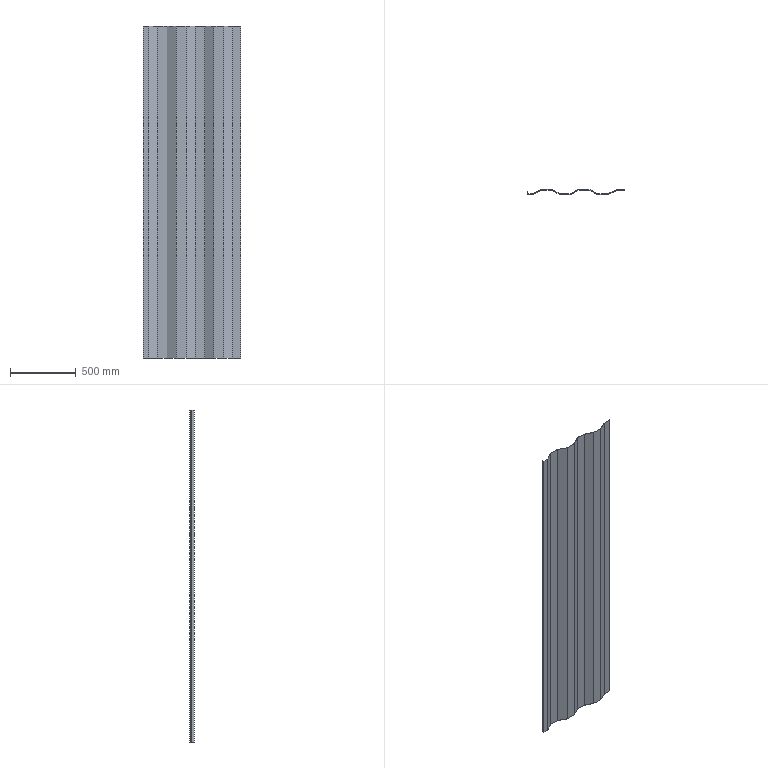Part | SolidWorks | features ExtruThin 1 | 1 solid | 28 faces | box 742 x 37.696 x 2530 mm | volume 4059329 mm3 | plane 28
STEP:
#1=CARTESIAN_POINT('',(679.865,31.696,0.));
#2=VERTEX_POINT('',#1);
#3=CARTESIAN_POINT('',(742.,31.696,0.));
#4=VERTEX_POINT('',#3);
#5=CARTESIAN_POINT('',(679.865,31.696,0.));
#6=DIRECTION('',(1.,0.,0.));
#7=VECTOR('',#6,1000.);
#8=LINE('',#5,#7);
#9=EDGE_CURVE('',#2,#4,#8,.T.);
#10=ORIENTED_EDGE('',*,*,#9,.T.);
#11=CARTESIAN_POINT('',(742.,31.696,2530.));
#12=VERTEX_POINT('',#11);
#13=CARTESIAN_POINT('',(742.,31.696,2530.));
#14=DIRECTION('',(0.,0.,-1.));
#15=VECTOR('',#14,1000.);
#16=LINE('',#13,#15);
#17=EDGE_CURVE('',#12,#4,#16,.T.);
#18=ORIENTED_EDGE('',*,*,#17,.F.);
#19=CARTESIAN_POINT('',(679.865,31.696,2530.));
#20=VERTEX_POINT('',#19);
#21=CARTESIAN_POINT('',(679.865,31.696,2530.));
#22=DIRECTION('',(1.,0.,0.));
#23=VECTOR('',#22,1000.);
#24=LINE('',#21,#23);
#25=EDGE_CURVE('',#20,#12,#24,.T.);
#26=ORIENTED_EDGE('',*,*,#25,.F.);
#27=CARTESIAN_POINT('',(679.865,31.696,2530.));
#28=DIRECTION('',(0.,0.,-1.));
#29=VECTOR('',#28,1000.);
#30=LINE('',#27,#29);
#31=EDGE_CURVE('',#20,#2,#30,.T.);
#32=ORIENTED_EDGE('',*,*,#31,.T.);
#33=EDGE_LOOP('',(#10,#18,#26,#32));
#34=FACE_OUTER_BOUND('',#33,.T.);
#35=CARTESIAN_POINT('',(679.865,31.696,2530.));
#36=DIRECTION('',(0.,1.,0.));
#37=DIRECTION('',(0.,0.,1.));
#38=AXIS2_PLACEMENT_3D('',#35,#36,#37);
#39=PLANE('',#38);
#40=ADVANCED_FACE('',(#34),#39,.F.);
#41=CARTESIAN_POINT('',(742.,33.696,0.));
#42=VERTEX_POINT('',#41);
#43=CARTESIAN_POINT('',(742.,33.696,0.));
#44=DIRECTION('',(0.,-1.,0.));
#45=VECTOR('',#44,1000.);
#46=LINE('',#43,#45);
#47=EDGE_CURVE('',#42,#4,#46,.T.);
#48=ORIENTED_EDGE('',*,*,#47,.F.);
#49=CARTESIAN_POINT('',(742.,33.696,2530.));
#50=VERTEX_POINT('',#49);
#51=CARTESIAN_POINT('',(742.,33.696,2530.));
#52=DIRECTION('',(0.,0.,-1.));
#53=VECTOR('',#52,1000.);
#54=LINE('',#51,#53);
#55=EDGE_CURVE('',#50,#42,#54,.T.);
#56=ORIENTED_EDGE('',*,*,#55,.F.);
#57=CARTESIAN_POINT('',(742.,33.696,2530.));
#58=DIRECTION('',(0.,-1.,0.));
#59=VECTOR('',#58,1000.);
#60=LINE('',#57,#59);
#61=EDGE_CURVE('',#50,#12,#60,.T.);
#62=ORIENTED_EDGE('',*,*,#61,.T.);
#63=ORIENTED_EDGE('',*,*,#17,.T.);
#64=EDGE_LOOP('',(#48,#56,#62,#63));
#65=FACE_OUTER_BOUND('',#64,.T.);
#66=CARTESIAN_POINT('',(742.,33.696,2530.));
#67=DIRECTION('',(1.,0.,0.));
#68=DIRECTION('',(0.,0.,-1.));
#69=AXIS2_PLACEMENT_3D('',#66,#67,#68);
#70=PLANE('',#69);
#71=ADVANCED_FACE('',(#65),#70,.T.);
#72=CARTESIAN_POINT('',(679.422,33.696,0.));
#73=VERTEX_POINT('',#72);
#74=CARTESIAN_POINT('',(679.865,33.696,0.));
#75=DIRECTION('',(1.,0.,0.));
#76=VECTOR('',#75,1000.);
#77=LINE('',#74,#76);
#78=EDGE_CURVE('',#73,#42,#77,.T.);
#79=ORIENTED_EDGE('',*,*,#78,.F.);
#80=CARTESIAN_POINT('',(679.422,33.696,2530.));
#81=VERTEX_POINT('',#80);
#82=CARTESIAN_POINT('',(679.422,33.696,2530.));
#83=DIRECTION('',(0.,0.,-1.));
#84=VECTOR('',#83,1000.);
#85=LINE('',#82,#84);
#86=EDGE_CURVE('',#81,#73,#85,.T.);
#87=ORIENTED_EDGE('',*,*,#86,.F.);
#88=CARTESIAN_POINT('',(679.865,33.696,2530.));
#89=DIRECTION('',(1.,0.,0.));
#90=VECTOR('',#89,1000.);
#91=LINE('',#88,#90);
#92=EDGE_CURVE('',#81,#50,#91,.T.);
#93=ORIENTED_EDGE('',*,*,#92,.T.);
#94=ORIENTED_EDGE('',*,*,#55,.T.);
#95=EDGE_LOOP('',(#79,#87,#93,#94));
#96=FACE_OUTER_BOUND('',#95,.T.);
#97=CARTESIAN_POINT('',(679.865,33.696,2530.));
#98=DIRECTION('',(0.,1.,0.));
#99=DIRECTION('',(0.,0.,1.));
#100=AXIS2_PLACEMENT_3D('',#97,#98,#99);
#101=PLANE('',#100);
#102=ADVANCED_FACE('',(#96),#101,.T.);
#103=CARTESIAN_POINT('',(611.449,2.,0.));
#104=VERTEX_POINT('',#103);
#105=CARTESIAN_POINT('',(611.047,1.813,0.));
#106=DIRECTION('',(0.9063,0.4226,0.));
#107=VECTOR('',#106,1000.);
#108=LINE('',#105,#107);
#109=EDGE_CURVE('',#104,#73,#108,.T.);
#110=ORIENTED_EDGE('',*,*,#109,.F.);
#111=CARTESIAN_POINT('',(611.449,2.,2530.));
#112=VERTEX_POINT('',#111);
#113=CARTESIAN_POINT('',(611.449,2.,2530.));
#114=DIRECTION('',(0.,0.,-1.));
#115=VECTOR('',#114,1000.);
#116=LINE('',#113,#115);
#117=EDGE_CURVE('',#112,#104,#116,.T.);
#118=ORIENTED_EDGE('',*,*,#117,.F.);
#119=CARTESIAN_POINT('',(611.047,1.813,2530.));
#120=DIRECTION('',(0.9063,0.4226,0.));
#121=VECTOR('',#120,1000.);
#122=LINE('',#119,#121);
#123=EDGE_CURVE('',#112,#81,#122,.T.);
#124=ORIENTED_EDGE('',*,*,#123,.T.);
#125=ORIENTED_EDGE('',*,*,#86,.T.);
#126=EDGE_LOOP('',(#110,#118,#124,#125));
#127=FACE_OUTER_BOUND('',#126,.T.);
#128=CARTESIAN_POINT('',(611.047,1.813,2530.));
#129=DIRECTION('',(-0.4226,0.9063,0.));
#130=DIRECTION('',(-0.9063,-0.4226,0.));
#131=AXIS2_PLACEMENT_3D('',#128,#129,#130);
#132=PLANE('',#131);
#133=ADVANCED_FACE('',(#127),#132,.T.);
#134=CARTESIAN_POINT('',(537.386,2.,0.));
#135=VERTEX_POINT('',#134);
#136=CARTESIAN_POINT('',(536.892,2.,0.));
#137=DIRECTION('',(1.,0.,0.));
#138=VECTOR('',#137,1000.);
#139=LINE('',#136,#138);
#140=EDGE_CURVE('',#135,#104,#139,.T.);
#141=ORIENTED_EDGE('',*,*,#140,.F.);
#142=CARTESIAN_POINT('',(537.386,2.,2530.));
#143=VERTEX_POINT('',#142);
#144=CARTESIAN_POINT('',(537.386,2.,2530.));
#145=DIRECTION('',(0.,0.,-1.));
#146=VECTOR('',#145,1000.);
#147=LINE('',#144,#146);
#148=EDGE_CURVE('',#143,#135,#147,.T.);
#149=ORIENTED_EDGE('',*,*,#148,.F.);
#150=CARTESIAN_POINT('',(536.892,2.,2530.));
#151=DIRECTION('',(1.,0.,0.));
#152=VECTOR('',#151,1000.);
#153=LINE('',#150,#152);
#154=EDGE_CURVE('',#143,#112,#153,.T.);
#155=ORIENTED_EDGE('',*,*,#154,.T.);
#156=ORIENTED_EDGE('',*,*,#117,.T.);
#157=EDGE_LOOP('',(#141,#149,#155,#156));
#158=FACE_OUTER_BOUND('',#157,.T.);
#159=CARTESIAN_POINT('',(536.892,2.,2530.));
#160=DIRECTION('',(0.,1.,0.));
#161=DIRECTION('',(0.,0.,1.));
#162=AXIS2_PLACEMENT_3D('',#159,#160,#161);
#163=PLANE('',#162);
#164=ADVANCED_FACE('',(#158),#163,.T.);
#165=CARTESIAN_POINT('',(469.412,37.696,0.));
#166=VERTEX_POINT('',#165);
#167=CARTESIAN_POINT('',(469.849,37.467,0.));
#168=DIRECTION('',(0.8853,-0.4649,0.));
#169=VECTOR('',#168,1000.);
#170=LINE('',#167,#169);
#171=EDGE_CURVE('',#166,#135,#170,.T.);
#172=ORIENTED_EDGE('',*,*,#171,.F.);
#173=CARTESIAN_POINT('',(469.412,37.696,2530.));
#174=VERTEX_POINT('',#173);
#175=CARTESIAN_POINT('',(469.412,37.696,2530.));
#176=DIRECTION('',(0.,0.,-1.));
#177=VECTOR('',#176,1000.);
#178=LINE('',#175,#177);
#179=EDGE_CURVE('',#174,#166,#178,.T.);
#180=ORIENTED_EDGE('',*,*,#179,.F.);
#181=CARTESIAN_POINT('',(469.849,37.467,2530.));
#182=DIRECTION('',(0.8853,-0.4649,0.));
#183=VECTOR('',#182,1000.);
#184=LINE('',#181,#183);
#185=EDGE_CURVE('',#174,#143,#184,.T.);
#186=ORIENTED_EDGE('',*,*,#185,.T.);
#187=ORIENTED_EDGE('',*,*,#148,.T.);
#188=EDGE_LOOP('',(#172,#180,#186,#187));
#189=FACE_OUTER_BOUND('',#188,.T.);
#190=CARTESIAN_POINT('',(469.849,37.467,2530.));
#191=DIRECTION('',(0.4649,0.8853,0.));
#192=DIRECTION('',(-0.8853,0.4649,0.));
#193=AXIS2_PLACEMENT_3D('',#190,#191,#192);
#194=PLANE('',#193);
#195=ADVANCED_FACE('',(#189),#194,.T.);
#196=CARTESIAN_POINT('',(393.426,37.696,0.));
#197=VERTEX_POINT('',#196);
#198=CARTESIAN_POINT('',(393.919,37.696,0.));
#199=DIRECTION('',(1.,0.,0.));
#200=VECTOR('',#199,1000.);
#201=LINE('',#198,#200);
#202=EDGE_CURVE('',#197,#166,#201,.T.);
#203=ORIENTED_EDGE('',*,*,#202,.F.);
#204=CARTESIAN_POINT('',(393.426,37.696,2530.));
#205=VERTEX_POINT('',#204);
#206=CARTESIAN_POINT('',(393.426,37.696,2530.));
#207=DIRECTION('',(0.,0.,-1.));
#208=VECTOR('',#207,1000.);
#209=LINE('',#206,#208);
#210=EDGE_CURVE('',#205,#197,#209,.T.);
#211=ORIENTED_EDGE('',*,*,#210,.F.);
#212=CARTESIAN_POINT('',(393.919,37.696,2530.));
#213=DIRECTION('',(1.,0.,0.));
#214=VECTOR('',#213,1000.);
#215=LINE('',#212,#214);
#216=EDGE_CURVE('',#205,#174,#215,.T.);
#217=ORIENTED_EDGE('',*,*,#216,.T.);
#218=ORIENTED_EDGE('',*,*,#179,.T.);
#219=EDGE_LOOP('',(#203,#211,#217,#218));
#220=FACE_OUTER_BOUND('',#219,.T.);
#221=CARTESIAN_POINT('',(393.919,37.696,2530.));
#222=DIRECTION('',(0.,1.,0.));
#223=DIRECTION('',(0.,0.,1.));
#224=AXIS2_PLACEMENT_3D('',#221,#222,#223);
#225=PLANE('',#224);
#226=ADVANCED_FACE('',(#220),#225,.T.);
#227=CARTESIAN_POINT('',(325.453,2.,0.));
#228=VERTEX_POINT('',#227);
#229=CARTESIAN_POINT('',(325.016,1.771,0.));
#230=DIRECTION('',(0.8853,0.4649,0.));
#231=VECTOR('',#230,1000.);
#232=LINE('',#229,#231);
#233=EDGE_CURVE('',#228,#197,#232,.T.);
#234=ORIENTED_EDGE('',*,*,#233,.F.);
#235=CARTESIAN_POINT('',(325.453,2.,2530.));
#236=VERTEX_POINT('',#235);
#237=CARTESIAN_POINT('',(325.453,2.,2530.));
#238=DIRECTION('',(0.,0.,-1.));
#239=VECTOR('',#238,1000.);
#240=LINE('',#237,#239);
#241=EDGE_CURVE('',#236,#228,#240,.T.);
#242=ORIENTED_EDGE('',*,*,#241,.F.);
#243=CARTESIAN_POINT('',(325.016,1.771,2530.));
#244=DIRECTION('',(0.8853,0.4649,0.));
#245=VECTOR('',#244,1000.);
#246=LINE('',#243,#245);
#247=EDGE_CURVE('',#236,#205,#246,.T.);
#248=ORIENTED_EDGE('',*,*,#247,.T.);
#249=ORIENTED_EDGE('',*,*,#210,.T.);
#250=EDGE_LOOP('',(#234,#242,#248,#249));
#251=FACE_OUTER_BOUND('',#250,.T.);
#252=CARTESIAN_POINT('',(325.016,1.771,2530.));
#253=DIRECTION('',(-0.4649,0.8853,0.));
#254=DIRECTION('',(-0.8853,-0.4649,0.));
#255=AXIS2_PLACEMENT_3D('',#252,#253,#254);
#256=PLANE('',#255);
#257=ADVANCED_FACE('',(#251),#256,.T.);
#258=CARTESIAN_POINT('',(251.439,2.,0.));
#259=VERTEX_POINT('',#258);
#260=CARTESIAN_POINT('',(250.946,2.,0.));
#261=DIRECTION('',(1.,0.,0.));
#262=VECTOR('',#261,1000.);
#263=LINE('',#260,#262);
#264=EDGE_CURVE('',#259,#228,#263,.T.);
#265=ORIENTED_EDGE('',*,*,#264,.F.);
#266=CARTESIAN_POINT('',(251.439,2.,2530.));
#267=VERTEX_POINT('',#266);
#268=CARTESIAN_POINT('',(251.439,2.,2530.));
#269=DIRECTION('',(0.,0.,-1.));
#270=VECTOR('',#269,1000.);
#271=LINE('',#268,#270);
#272=EDGE_CURVE('',#267,#259,#271,.T.);
#273=ORIENTED_EDGE('',*,*,#272,.F.);
#274=CARTESIAN_POINT('',(250.946,2.,2530.));
#275=DIRECTION('',(1.,0.,0.));
#276=VECTOR('',#275,1000.);
#277=LINE('',#274,#276);
#278=EDGE_CURVE('',#267,#236,#277,.T.);
#279=ORIENTED_EDGE('',*,*,#278,.T.);
#280=ORIENTED_EDGE('',*,*,#241,.T.);
#281=EDGE_LOOP('',(#265,#273,#279,#280));
#282=FACE_OUTER_BOUND('',#281,.T.);
#283=CARTESIAN_POINT('',(250.946,2.,2530.));
#284=DIRECTION('',(0.,1.,0.));
#285=DIRECTION('',(0.,0.,1.));
#286=AXIS2_PLACEMENT_3D('',#283,#284,#285);
#287=PLANE('',#286);
#288=ADVANCED_FACE('',(#282),#287,.T.);
#289=CARTESIAN_POINT('',(183.466,37.696,0.));
#290=VERTEX_POINT('',#289);
#291=CARTESIAN_POINT('',(183.903,37.467,0.));
#292=DIRECTION('',(0.8853,-0.4649,0.));
#293=VECTOR('',#292,1000.);
#294=LINE('',#291,#293);
#295=EDGE_CURVE('',#290,#259,#294,.T.);
#296=ORIENTED_EDGE('',*,*,#295,.F.);
#297=CARTESIAN_POINT('',(183.466,37.696,2530.));
#298=VERTEX_POINT('',#297);
#299=CARTESIAN_POINT('',(183.466,37.696,2530.));
#300=DIRECTION('',(0.,0.,-1.));
#301=VECTOR('',#300,1000.);
#302=LINE('',#299,#301);
#303=EDGE_CURVE('',#298,#290,#302,.T.);
#304=ORIENTED_EDGE('',*,*,#303,.F.);
#305=CARTESIAN_POINT('',(183.903,37.467,2530.));
#306=DIRECTION('',(0.8853,-0.4649,0.));
#307=VECTOR('',#306,1000.);
#308=LINE('',#305,#307);
#309=EDGE_CURVE('',#298,#267,#308,.T.);
#310=ORIENTED_EDGE('',*,*,#309,.T.);
#311=ORIENTED_EDGE('',*,*,#272,.T.);
#312=EDGE_LOOP('',(#296,#304,#310,#311));
#313=FACE_OUTER_BOUND('',#312,.T.);
#314=CARTESIAN_POINT('',(183.903,37.467,2530.));
#315=DIRECTION('',(0.4649,0.8853,0.));
#316=DIRECTION('',(-0.8853,0.4649,0.));
#317=AXIS2_PLACEMENT_3D('',#314,#315,#316);
#318=PLANE('',#317);
#319=ADVANCED_FACE('',(#313),#318,.T.);
#320=CARTESIAN_POINT('',(107.48,37.696,0.));
#321=VERTEX_POINT('',#320);
#322=CARTESIAN_POINT('',(107.973,37.696,0.));
#323=DIRECTION('',(1.,0.,0.));
#324=VECTOR('',#323,1000.);
#325=LINE('',#322,#324);
#326=EDGE_CURVE('',#321,#290,#325,.T.);
#327=ORIENTED_EDGE('',*,*,#326,.F.);
#328=CARTESIAN_POINT('',(107.48,37.696,2530.));
#329=VERTEX_POINT('',#328);
#330=CARTESIAN_POINT('',(107.48,37.696,2530.));
#331=DIRECTION('',(0.,0.,-1.));
#332=VECTOR('',#331,1000.);
#333=LINE('',#330,#332);
#334=EDGE_CURVE('',#329,#321,#333,.T.);
#335=ORIENTED_EDGE('',*,*,#334,.F.);
#336=CARTESIAN_POINT('',(107.973,37.696,2530.));
#337=DIRECTION('',(1.,0.,0.));
#338=VECTOR('',#337,1000.);
#339=LINE('',#336,#338);
#340=EDGE_CURVE('',#329,#298,#339,.T.);
#341=ORIENTED_EDGE('',*,*,#340,.T.);
#342=ORIENTED_EDGE('',*,*,#303,.T.);
#343=EDGE_LOOP('',(#327,#335,#341,#342));
#344=FACE_OUTER_BOUND('',#343,.T.);
#345=CARTESIAN_POINT('',(107.973,37.696,2530.));
#346=DIRECTION('',(0.,1.,0.));
#347=DIRECTION('',(0.,0.,1.));
#348=AXIS2_PLACEMENT_3D('',#345,#346,#347);
#349=PLANE('',#348);
#350=ADVANCED_FACE('',(#344),#349,.T.);
#351=CARTESIAN_POINT('',(39.507,2.,0.));
#352=VERTEX_POINT('',#351);
#353=CARTESIAN_POINT('',(39.07,1.771,0.));
#354=DIRECTION('',(0.8853,0.4649,0.));
#355=VECTOR('',#354,1000.);
#356=LINE('',#353,#355);
#357=EDGE_CURVE('',#352,#321,#356,.T.);
#358=ORIENTED_EDGE('',*,*,#357,.F.);
#359=CARTESIAN_POINT('',(39.507,2.,2530.));
#360=VERTEX_POINT('',#359);
#361=CARTESIAN_POINT('',(39.507,2.,2530.));
#362=DIRECTION('',(0.,0.,-1.));
#363=VECTOR('',#362,1000.);
#364=LINE('',#361,#363);
#365=EDGE_CURVE('',#360,#352,#364,.T.);
#366=ORIENTED_EDGE('',*,*,#365,.F.);
#367=CARTESIAN_POINT('',(39.07,1.771,2530.));
#368=DIRECTION('',(0.8853,0.4649,0.));
#369=VECTOR('',#368,1000.);
#370=LINE('',#367,#369);
#371=EDGE_CURVE('',#360,#329,#370,.T.);
#372=ORIENTED_EDGE('',*,*,#371,.T.);
#373=ORIENTED_EDGE('',*,*,#334,.T.);
#374=EDGE_LOOP('',(#358,#366,#372,#373));
#375=FACE_OUTER_BOUND('',#374,.T.);
#376=CARTESIAN_POINT('',(39.07,1.771,2530.));
#377=DIRECTION('',(-0.4649,0.8853,0.));
#378=DIRECTION('',(-0.8853,-0.4649,0.));
#379=AXIS2_PLACEMENT_3D('',#376,#377,#378);
#380=PLANE('',#379);
#381=ADVANCED_FACE('',(#375),#380,.T.);
#382=CARTESIAN_POINT('',(2.,2.,0.));
#383=VERTEX_POINT('',#382);
#384=CARTESIAN_POINT('',(0.,2.,0.));
#385=DIRECTION('',(1.,0.,0.));
#386=VECTOR('',#385,1000.);
#387=LINE('',#384,#386);
#388=EDGE_CURVE('',#383,#352,#387,.T.);
#389=ORIENTED_EDGE('',*,*,#388,.F.);
#390=CARTESIAN_POINT('',(2.,2.,2530.));
#391=VERTEX_POINT('',#390);
#392=CARTESIAN_POINT('',(2.,2.,2530.));
#393=DIRECTION('',(0.,0.,-1.));
#394=VECTOR('',#393,1000.);
#395=LINE('',#392,#394);
#396=EDGE_CURVE('',#391,#383,#395,.T.);
#397=ORIENTED_EDGE('',*,*,#396,.F.);
#398=CARTESIAN_POINT('',(0.,2.,2530.));
#399=DIRECTION('',(1.,0.,0.));
#400=VECTOR('',#399,1000.);
#401=LINE('',#398,#400);
#402=EDGE_CURVE('',#391,#360,#401,.T.);
#403=ORIENTED_EDGE('',*,*,#402,.T.);
#404=ORIENTED_EDGE('',*,*,#365,.T.);
#405=EDGE_LOOP('',(#389,#397,#403,#404));
#406=FACE_OUTER_BOUND('',#405,.T.);
#407=CARTESIAN_POINT('',(0.,2.,2530.));
#408=DIRECTION('',(0.,1.,0.));
#409=DIRECTION('',(0.,0.,1.));
#410=AXIS2_PLACEMENT_3D('',#407,#408,#409);
#411=PLANE('',#410);
#412=ADVANCED_FACE('',(#406),#411,.T.);
#413=CARTESIAN_POINT('',(2.,20.,0.));
#414=VERTEX_POINT('',#413);
#415=CARTESIAN_POINT('',(2.,20.,0.));
#416=DIRECTION('',(0.,-1.,0.));
#417=VECTOR('',#416,1000.);
#418=LINE('',#415,#417);
#419=EDGE_CURVE('',#414,#383,#418,.T.);
#420=ORIENTED_EDGE('',*,*,#419,.F.);
#421=CARTESIAN_POINT('',(2.,20.,2530.));
#422=VERTEX_POINT('',#421);
#423=CARTESIAN_POINT('',(2.,20.,2530.));
#424=DIRECTION('',(0.,0.,-1.));
#425=VECTOR('',#424,1000.);
#426=LINE('',#423,#425);
#427=EDGE_CURVE('',#422,#414,#426,.T.);
#428=ORIENTED_EDGE('',*,*,#427,.F.);
#429=CARTESIAN_POINT('',(2.,20.,2530.));
#430=DIRECTION('',(0.,-1.,0.));
#431=VECTOR('',#430,1000.);
#432=LINE('',#429,#431);
#433=EDGE_CURVE('',#422,#391,#432,.T.);
#434=ORIENTED_EDGE('',*,*,#433,.T.);
#435=ORIENTED_EDGE('',*,*,#396,.T.);
#436=EDGE_LOOP('',(#420,#428,#434,#435));
#437=FACE_OUTER_BOUND('',#436,.T.);
#438=CARTESIAN_POINT('',(2.,20.,2530.));
#439=DIRECTION('',(1.,0.,0.));
#440=DIRECTION('',(0.,0.,-1.));
#441=AXIS2_PLACEMENT_3D('',#438,#439,#440);
#442=PLANE('',#441);
#443=ADVANCED_FACE('',(#437),#442,.T.);
#444=CARTESIAN_POINT('',(0.,20.,0.));
#445=VERTEX_POINT('',#444);
#446=CARTESIAN_POINT('',(0.,20.,0.));
#447=DIRECTION('',(1.,0.,0.));
#448=VECTOR('',#447,1000.);
#449=LINE('',#446,#448);
#450=EDGE_CURVE('',#445,#414,#449,.T.);
#451=ORIENTED_EDGE('',*,*,#450,.F.);
#452=CARTESIAN_POINT('',(0.,20.,2530.));
#453=VERTEX_POINT('',#452);
#454=CARTESIAN_POINT('',(0.,20.,2530.));
#455=DIRECTION('',(0.,0.,-1.));
#456=VECTOR('',#455,1000.);
#457=LINE('',#454,#456);
#458=EDGE_CURVE('',#453,#445,#457,.T.);
#459=ORIENTED_EDGE('',*,*,#458,.F.);
#460=CARTESIAN_POINT('',(0.,20.,2530.));
#461=DIRECTION('',(1.,0.,0.));
#462=VECTOR('',#461,1000.);
#463=LINE('',#460,#462);
#464=EDGE_CURVE('',#453,#422,#463,.T.);
#465=ORIENTED_EDGE('',*,*,#464,.T.);
#466=ORIENTED_EDGE('',*,*,#427,.T.);
#467=EDGE_LOOP('',(#451,#459,#465,#466));
#468=FACE_OUTER_BOUND('',#467,.T.);
#469=CARTESIAN_POINT('',(0.,20.,2530.));
#470=DIRECTION('',(0.,1.,0.));
#471=DIRECTION('',(0.,0.,1.));
#472=AXIS2_PLACEMENT_3D('',#469,#470,#471);
#473=PLANE('',#472);
#474=ADVANCED_FACE('',(#468),#473,.T.);
#475=CARTESIAN_POINT('',(0.,0.,0.));
#476=VERTEX_POINT('',#475);
#477=CARTESIAN_POINT('',(0.,20.,0.));
#478=DIRECTION('',(0.,-1.,0.));
#479=VECTOR('',#478,1000.);
#480=LINE('',#477,#479);
#481=EDGE_CURVE('',#445,#476,#480,.T.);
#482=ORIENTED_EDGE('',*,*,#481,.T.);
#483=CARTESIAN_POINT('',(0.,0.,2530.));
#484=VERTEX_POINT('',#483);
#485=CARTESIAN_POINT('',(0.,0.,2530.));
#486=DIRECTION('',(0.,0.,-1.));
#487=VECTOR('',#486,1000.);
#488=LINE('',#485,#487);
#489=EDGE_CURVE('',#484,#476,#488,.T.);
#490=ORIENTED_EDGE('',*,*,#489,.F.);
#491=CARTESIAN_POINT('',(0.,20.,2530.));
#492=DIRECTION('',(0.,-1.,0.));
#493=VECTOR('',#492,1000.);
#494=LINE('',#491,#493);
#495=EDGE_CURVE('',#453,#484,#494,.T.);
#496=ORIENTED_EDGE('',*,*,#495,.F.);
#497=ORIENTED_EDGE('',*,*,#458,.T.);
#498=EDGE_LOOP('',(#482,#490,#496,#497));
#499=FACE_OUTER_BOUND('',#498,.T.);
#500=CARTESIAN_POINT('',(0.,20.,2530.));
#501=DIRECTION('',(1.,0.,0.));
#502=DIRECTION('',(0.,0.,-1.));
#503=AXIS2_PLACEMENT_3D('',#500,#501,#502);
#504=PLANE('',#503);
#505=ADVANCED_FACE('',(#499),#504,.F.);
#506=CARTESIAN_POINT('',(40.,0.,0.));
#507=VERTEX_POINT('',#506);
#508=CARTESIAN_POINT('',(0.,0.,0.));
#509=DIRECTION('',(1.,0.,0.));
#510=VECTOR('',#509,1000.);
#511=LINE('',#508,#510);
#512=EDGE_CURVE('',#476,#507,#511,.T.);
#513=ORIENTED_EDGE('',*,*,#512,.T.);
#514=CARTESIAN_POINT('',(40.,0.,2530.));
#515=VERTEX_POINT('',#514);
#516=CARTESIAN_POINT('',(40.,0.,2530.));
#517=DIRECTION('',(0.,0.,-1.));
#518=VECTOR('',#517,1000.);
#519=LINE('',#516,#518);
#520=EDGE_CURVE('',#515,#507,#519,.T.);
#521=ORIENTED_EDGE('',*,*,#520,.F.);
#522=CARTESIAN_POINT('',(0.,0.,2530.));
#523=DIRECTION('',(1.,0.,0.));
#524=VECTOR('',#523,1000.);
#525=LINE('',#522,#524);
#526=EDGE_CURVE('',#484,#515,#525,.T.);
#527=ORIENTED_EDGE('',*,*,#526,.F.);
#528=ORIENTED_EDGE('',*,*,#489,.T.);
#529=EDGE_LOOP('',(#513,#521,#527,#528));
#530=FACE_OUTER_BOUND('',#529,.T.);
#531=CARTESIAN_POINT('',(0.,0.,2530.));
#532=DIRECTION('',(0.,1.,0.));
#533=DIRECTION('',(0.,0.,1.));
#534=AXIS2_PLACEMENT_3D('',#531,#532,#533);
#535=PLANE('',#534);
#536=ADVANCED_FACE('',(#530),#535,.F.);
#537=CARTESIAN_POINT('',(107.973,35.696,0.));
#538=VERTEX_POINT('',#537);
#539=CARTESIAN_POINT('',(40.,0.,0.));
#540=DIRECTION('',(0.8853,0.4649,0.));
#541=VECTOR('',#540,1000.);
#542=LINE('',#539,#541);
#543=EDGE_CURVE('',#507,#538,#542,.T.);
#544=ORIENTED_EDGE('',*,*,#543,.T.);
#545=CARTESIAN_POINT('',(107.973,35.696,2530.));
#546=VERTEX_POINT('',#545);
#547=CARTESIAN_POINT('',(107.973,35.696,2530.));
#548=DIRECTION('',(0.,0.,-1.));
#549=VECTOR('',#548,1000.);
#550=LINE('',#547,#549);
#551=EDGE_CURVE('',#546,#538,#550,.T.);
#552=ORIENTED_EDGE('',*,*,#551,.F.);
#553=CARTESIAN_POINT('',(40.,0.,2530.));
#554=DIRECTION('',(0.8853,0.4649,0.));
#555=VECTOR('',#554,1000.);
#556=LINE('',#553,#555);
#557=EDGE_CURVE('',#515,#546,#556,.T.);
#558=ORIENTED_EDGE('',*,*,#557,.F.);
#559=ORIENTED_EDGE('',*,*,#520,.T.);
#560=EDGE_LOOP('',(#544,#552,#558,#559));
#561=FACE_OUTER_BOUND('',#560,.T.);
#562=CARTESIAN_POINT('',(40.,0.,2530.));
#563=DIRECTION('',(-0.4649,0.8853,0.));
#564=DIRECTION('',(-0.8853,-0.4649,0.));
#565=AXIS2_PLACEMENT_3D('',#562,#563,#564);
#566=PLANE('',#565);
#567=ADVANCED_FACE('',(#561),#566,.F.);
#568=CARTESIAN_POINT('',(182.973,35.696,0.));
#569=VERTEX_POINT('',#568);
#570=CARTESIAN_POINT('',(107.973,35.696,0.));
#571=DIRECTION('',(1.,0.,0.));
#572=VECTOR('',#571,1000.);
#573=LINE('',#570,#572);
#574=EDGE_CURVE('',#538,#569,#573,.T.);
#575=ORIENTED_EDGE('',*,*,#574,.T.);
#576=CARTESIAN_POINT('',(182.973,35.696,2530.));
#577=VERTEX_POINT('',#576);
#578=CARTESIAN_POINT('',(182.973,35.696,2530.));
#579=DIRECTION('',(0.,0.,-1.));
#580=VECTOR('',#579,1000.);
#581=LINE('',#578,#580);
#582=EDGE_CURVE('',#577,#569,#581,.T.);
#583=ORIENTED_EDGE('',*,*,#582,.F.);
#584=CARTESIAN_POINT('',(107.973,35.696,2530.));
#585=DIRECTION('',(1.,0.,0.));
#586=VECTOR('',#585,1000.);
#587=LINE('',#584,#586);
#588=EDGE_CURVE('',#546,#577,#587,.T.);
#589=ORIENTED_EDGE('',*,*,#588,.F.);
#590=ORIENTED_EDGE('',*,*,#551,.T.);
#591=EDGE_LOOP('',(#575,#583,#589,#590));
#592=FACE_OUTER_BOUND('',#591,.T.);
#593=CARTESIAN_POINT('',(107.973,35.696,2530.));
#594=DIRECTION('',(0.,1.,0.));
#595=DIRECTION('',(0.,0.,1.));
#596=AXIS2_PLACEMENT_3D('',#593,#594,#595);
#597=PLANE('',#596);
#598=ADVANCED_FACE('',(#592),#597,.F.);
#599=CARTESIAN_POINT('',(250.946,0.,0.));
#600=VERTEX_POINT('',#599);
#601=CARTESIAN_POINT('',(182.973,35.696,0.));
#602=DIRECTION('',(0.8853,-0.4649,0.));
#603=VECTOR('',#602,1000.);
#604=LINE('',#601,#603);
#605=EDGE_CURVE('',#569,#600,#604,.T.);
#606=ORIENTED_EDGE('',*,*,#605,.T.);
#607=CARTESIAN_POINT('',(250.946,0.,2530.));
#608=VERTEX_POINT('',#607);
#609=CARTESIAN_POINT('',(250.946,0.,2530.));
#610=DIRECTION('',(0.,0.,-1.));
#611=VECTOR('',#610,1000.);
#612=LINE('',#609,#611);
#613=EDGE_CURVE('',#608,#600,#612,.T.);
#614=ORIENTED_EDGE('',*,*,#613,.F.);
#615=CARTESIAN_POINT('',(182.973,35.696,2530.));
#616=DIRECTION('',(0.8853,-0.4649,0.));
#617=VECTOR('',#616,1000.);
#618=LINE('',#615,#617);
#619=EDGE_CURVE('',#577,#608,#618,.T.);
#620=ORIENTED_EDGE('',*,*,#619,.F.);
#621=ORIENTED_EDGE('',*,*,#582,.T.);
#622=EDGE_LOOP('',(#606,#614,#620,#621));
#623=FACE_OUTER_BOUND('',#622,.T.);
#624=CARTESIAN_POINT('',(182.973,35.696,2530.));
#625=DIRECTION('',(0.4649,0.8853,0.));
#626=DIRECTION('',(-0.8853,0.4649,0.));
#627=AXIS2_PLACEMENT_3D('',#624,#625,#626);
#628=PLANE('',#627);
#629=ADVANCED_FACE('',(#623),#628,.F.);
#630=CARTESIAN_POINT('',(325.946,0.,0.));
#631=VERTEX_POINT('',#630);
#632=CARTESIAN_POINT('',(250.946,0.,0.));
#633=DIRECTION('',(1.,0.,0.));
#634=VECTOR('',#633,1000.);
#635=LINE('',#632,#634);
#636=EDGE_CURVE('',#600,#631,#635,.T.);
#637=ORIENTED_EDGE('',*,*,#636,.T.);
#638=CARTESIAN_POINT('',(325.946,0.,2530.));
#639=VERTEX_POINT('',#638);
#640=CARTESIAN_POINT('',(325.946,0.,2530.));
#641=DIRECTION('',(0.,0.,-1.));
#642=VECTOR('',#641,1000.);
#643=LINE('',#640,#642);
#644=EDGE_CURVE('',#639,#631,#643,.T.);
#645=ORIENTED_EDGE('',*,*,#644,.F.);
#646=CARTESIAN_POINT('',(250.946,0.,2530.));
#647=DIRECTION('',(1.,0.,0.));
#648=VECTOR('',#647,1000.);
#649=LINE('',#646,#648);
#650=EDGE_CURVE('',#608,#639,#649,.T.);
#651=ORIENTED_EDGE('',*,*,#650,.F.);
#652=ORIENTED_EDGE('',*,*,#613,.T.);
#653=EDGE_LOOP('',(#637,#645,#651,#652));
#654=FACE_OUTER_BOUND('',#653,.T.);
#655=CARTESIAN_POINT('',(250.946,0.,2530.));
#656=DIRECTION('',(0.,1.,0.));
#657=DIRECTION('',(0.,0.,1.));
#658=AXIS2_PLACEMENT_3D('',#655,#656,#657);
#659=PLANE('',#658);
#660=ADVANCED_FACE('',(#654),#659,.F.);
#661=CARTESIAN_POINT('',(393.919,35.696,0.));
#662=VERTEX_POINT('',#661);
#663=CARTESIAN_POINT('',(325.946,0.,0.));
#664=DIRECTION('',(0.8853,0.4649,0.));
#665=VECTOR('',#664,1000.);
#666=LINE('',#663,#665);
#667=EDGE_CURVE('',#631,#662,#666,.T.);
#668=ORIENTED_EDGE('',*,*,#667,.T.);
#669=CARTESIAN_POINT('',(393.919,35.696,2530.));
#670=VERTEX_POINT('',#669);
#671=CARTESIAN_POINT('',(393.919,35.696,2530.));
#672=DIRECTION('',(0.,0.,-1.));
#673=VECTOR('',#672,1000.);
#674=LINE('',#671,#673);
#675=EDGE_CURVE('',#670,#662,#674,.T.);
#676=ORIENTED_EDGE('',*,*,#675,.F.);
#677=CARTESIAN_POINT('',(325.946,0.,2530.));
#678=DIRECTION('',(0.8853,0.4649,0.));
#679=VECTOR('',#678,1000.);
#680=LINE('',#677,#679);
#681=EDGE_CURVE('',#639,#670,#680,.T.);
#682=ORIENTED_EDGE('',*,*,#681,.F.);
#683=ORIENTED_EDGE('',*,*,#644,.T.);
#684=EDGE_LOOP('',(#668,#676,#682,#683));
#685=FACE_OUTER_BOUND('',#684,.T.);
#686=CARTESIAN_POINT('',(325.946,0.,2530.));
#687=DIRECTION('',(-0.4649,0.8853,0.));
#688=DIRECTION('',(-0.8853,-0.4649,0.));
#689=AXIS2_PLACEMENT_3D('',#686,#687,#688);
#690=PLANE('',#689);
#691=ADVANCED_FACE('',(#685),#690,.F.);
#692=CARTESIAN_POINT('',(468.919,35.696,0.));
#693=VERTEX_POINT('',#692);
#694=CARTESIAN_POINT('',(393.919,35.696,0.));
#695=DIRECTION('',(1.,0.,0.));
#696=VECTOR('',#695,1000.);
#697=LINE('',#694,#696);
#698=EDGE_CURVE('',#662,#693,#697,.T.);
#699=ORIENTED_EDGE('',*,*,#698,.T.);
#700=CARTESIAN_POINT('',(468.919,35.696,2530.));
#701=VERTEX_POINT('',#700);
#702=CARTESIAN_POINT('',(468.919,35.696,2530.));
#703=DIRECTION('',(0.,0.,-1.));
#704=VECTOR('',#703,1000.);
#705=LINE('',#702,#704);
#706=EDGE_CURVE('',#701,#693,#705,.T.);
#707=ORIENTED_EDGE('',*,*,#706,.F.);
#708=CARTESIAN_POINT('',(393.919,35.696,2530.));
#709=DIRECTION('',(1.,0.,0.));
#710=VECTOR('',#709,1000.);
#711=LINE('',#708,#710);
#712=EDGE_CURVE('',#670,#701,#711,.T.);
#713=ORIENTED_EDGE('',*,*,#712,.F.);
#714=ORIENTED_EDGE('',*,*,#675,.T.);
#715=EDGE_LOOP('',(#699,#707,#713,#714));
#716=FACE_OUTER_BOUND('',#715,.T.);
#717=CARTESIAN_POINT('',(393.919,35.696,2530.));
#718=DIRECTION('',(0.,1.,0.));
#719=DIRECTION('',(0.,0.,1.));
#720=AXIS2_PLACEMENT_3D('',#717,#718,#719);
#721=PLANE('',#720);
#722=ADVANCED_FACE('',(#716),#721,.F.);
#723=CARTESIAN_POINT('',(536.892,0.,0.));
#724=VERTEX_POINT('',#723);
#725=CARTESIAN_POINT('',(468.919,35.696,0.));
#726=DIRECTION('',(0.8853,-0.4649,0.));
#727=VECTOR('',#726,1000.);
#728=LINE('',#725,#727);
#729=EDGE_CURVE('',#693,#724,#728,.T.);
#730=ORIENTED_EDGE('',*,*,#729,.T.);
#731=CARTESIAN_POINT('',(536.892,0.,2530.));
#732=VERTEX_POINT('',#731);
#733=CARTESIAN_POINT('',(536.892,0.,2530.));
#734=DIRECTION('',(0.,0.,-1.));
#735=VECTOR('',#734,1000.);
#736=LINE('',#733,#735);
#737=EDGE_CURVE('',#732,#724,#736,.T.);
#738=ORIENTED_EDGE('',*,*,#737,.F.);
#739=CARTESIAN_POINT('',(468.919,35.696,2530.));
#740=DIRECTION('',(0.8853,-0.4649,0.));
#741=VECTOR('',#740,1000.);
#742=LINE('',#739,#741);
#743=EDGE_CURVE('',#701,#732,#742,.T.);
#744=ORIENTED_EDGE('',*,*,#743,.F.);
#745=ORIENTED_EDGE('',*,*,#706,.T.);
#746=EDGE_LOOP('',(#730,#738,#744,#745));
#747=FACE_OUTER_BOUND('',#746,.T.);
#748=CARTESIAN_POINT('',(468.919,35.696,2530.));
#749=DIRECTION('',(0.4649,0.8853,0.));
#750=DIRECTION('',(-0.8853,0.4649,0.));
#751=AXIS2_PLACEMENT_3D('',#748,#749,#750);
#752=PLANE('',#751);
#753=ADVANCED_FACE('',(#747),#752,.F.);
#754=CARTESIAN_POINT('',(611.892,0.,0.));
#755=VERTEX_POINT('',#754);
#756=CARTESIAN_POINT('',(536.892,0.,0.));
#757=DIRECTION('',(1.,0.,0.));
#758=VECTOR('',#757,1000.);
#759=LINE('',#756,#758);
#760=EDGE_CURVE('',#724,#755,#759,.T.);
#761=ORIENTED_EDGE('',*,*,#760,.T.);
#762=CARTESIAN_POINT('',(611.892,0.,2530.));
#763=VERTEX_POINT('',#762);
#764=CARTESIAN_POINT('',(611.892,0.,2530.));
#765=DIRECTION('',(0.,0.,-1.));
#766=VECTOR('',#765,1000.);
#767=LINE('',#764,#766);
#768=EDGE_CURVE('',#763,#755,#767,.T.);
#769=ORIENTED_EDGE('',*,*,#768,.F.);
#770=CARTESIAN_POINT('',(536.892,0.,2530.));
#771=DIRECTION('',(1.,0.,0.));
#772=VECTOR('',#771,1000.);
#773=LINE('',#770,#772);
#774=EDGE_CURVE('',#732,#763,#773,.T.);
#775=ORIENTED_EDGE('',*,*,#774,.F.);
#776=ORIENTED_EDGE('',*,*,#737,.T.);
#777=EDGE_LOOP('',(#761,#769,#775,#776));
#778=FACE_OUTER_BOUND('',#777,.T.);
#779=CARTESIAN_POINT('',(536.892,0.,2530.));
#780=DIRECTION('',(0.,1.,0.));
#781=DIRECTION('',(0.,0.,1.));
#782=AXIS2_PLACEMENT_3D('',#779,#780,#781);
#783=PLANE('',#782);
#784=ADVANCED_FACE('',(#778),#783,.F.);
#785=CARTESIAN_POINT('',(611.892,0.,0.));
#786=DIRECTION('',(0.9063,0.4226,0.));
#787=VECTOR('',#786,1000.);
#788=LINE('',#785,#787);
#789=EDGE_CURVE('',#755,#2,#788,.T.);
#790=ORIENTED_EDGE('',*,*,#789,.T.);
#791=ORIENTED_EDGE('',*,*,#31,.F.);
#792=CARTESIAN_POINT('',(611.892,0.,2530.));
#793=DIRECTION('',(0.9063,0.4226,0.));
#794=VECTOR('',#793,1000.);
#795=LINE('',#792,#794);
#796=EDGE_CURVE('',#763,#20,#795,.T.);
#797=ORIENTED_EDGE('',*,*,#796,.F.);
#798=ORIENTED_EDGE('',*,*,#768,.T.);
#799=EDGE_LOOP('',(#790,#791,#797,#798));
#800=FACE_OUTER_BOUND('',#799,.T.);
#801=CARTESIAN_POINT('',(611.892,0.,2530.));
#802=DIRECTION('',(-0.4226,0.9063,0.));
#803=DIRECTION('',(-0.9063,-0.4226,0.));
#804=AXIS2_PLACEMENT_3D('',#801,#802,#803);
#805=PLANE('',#804);
#806=ADVANCED_FACE('',(#800),#805,.F.);
#807=ORIENTED_EDGE('',*,*,#25,.T.);
#808=ORIENTED_EDGE('',*,*,#61,.F.);
#809=ORIENTED_EDGE('',*,*,#92,.F.);
#810=ORIENTED_EDGE('',*,*,#123,.F.);
#811=ORIENTED_EDGE('',*,*,#154,.F.);
#812=ORIENTED_EDGE('',*,*,#185,.F.);
#813=ORIENTED_EDGE('',*,*,#216,.F.);
#814=ORIENTED_EDGE('',*,*,#247,.F.);
#815=ORIENTED_EDGE('',*,*,#278,.F.);
#816=ORIENTED_EDGE('',*,*,#309,.F.);
#817=ORIENTED_EDGE('',*,*,#340,.F.);
#818=ORIENTED_EDGE('',*,*,#371,.F.);
#819=ORIENTED_EDGE('',*,*,#402,.F.);
#820=ORIENTED_EDGE('',*,*,#433,.F.);
#821=ORIENTED_EDGE('',*,*,#464,.F.);
#822=ORIENTED_EDGE('',*,*,#495,.T.);
#823=ORIENTED_EDGE('',*,*,#526,.T.);
#824=ORIENTED_EDGE('',*,*,#557,.T.);
#825=ORIENTED_EDGE('',*,*,#588,.T.);
#826=ORIENTED_EDGE('',*,*,#619,.T.);
#827=ORIENTED_EDGE('',*,*,#650,.T.);
#828=ORIENTED_EDGE('',*,*,#681,.T.);
#829=ORIENTED_EDGE('',*,*,#712,.T.);
#830=ORIENTED_EDGE('',*,*,#743,.T.);
#831=ORIENTED_EDGE('',*,*,#774,.T.);
#832=ORIENTED_EDGE('',*,*,#796,.T.);
#833=EDGE_LOOP('',(#807,#808,#809,#810,#811,#812,#813,#814,#815,#816,#817,#818,#819,#820,#821,#822,#823,#824,#825,#826,#827,#828,#829,#830,#831,#832));
#834=FACE_OUTER_BOUND('',#833,.T.);
#835=CARTESIAN_POINT('',(0.,0.,2530.));
#836=DIRECTION('',(0.,0.,-1.));
#837=DIRECTION('',(-1.,0.,0.));
#838=AXIS2_PLACEMENT_3D('',#835,#836,#837);
#839=PLANE('',#838);
#840=ADVANCED_FACE('',(#834),#839,.F.);
#841=ORIENTED_EDGE('',*,*,#9,.F.);
#842=ORIENTED_EDGE('',*,*,#789,.F.);
#843=ORIENTED_EDGE('',*,*,#760,.F.);
#844=ORIENTED_EDGE('',*,*,#729,.F.);
#845=ORIENTED_EDGE('',*,*,#698,.F.);
#846=ORIENTED_EDGE('',*,*,#667,.F.);
#847=ORIENTED_EDGE('',*,*,#636,.F.);
#848=ORIENTED_EDGE('',*,*,#605,.F.);
#849=ORIENTED_EDGE('',*,*,#574,.F.);
#850=ORIENTED_EDGE('',*,*,#543,.F.);
#851=ORIENTED_EDGE('',*,*,#512,.F.);
#852=ORIENTED_EDGE('',*,*,#481,.F.);
#853=ORIENTED_EDGE('',*,*,#450,.T.);
#854=ORIENTED_EDGE('',*,*,#419,.T.);
#855=ORIENTED_EDGE('',*,*,#388,.T.);
#856=ORIENTED_EDGE('',*,*,#357,.T.);
#857=ORIENTED_EDGE('',*,*,#326,.T.);
#858=ORIENTED_EDGE('',*,*,#295,.T.);
#859=ORIENTED_EDGE('',*,*,#264,.T.);
#860=ORIENTED_EDGE('',*,*,#233,.T.);
#861=ORIENTED_EDGE('',*,*,#202,.T.);
#862=ORIENTED_EDGE('',*,*,#171,.T.);
#863=ORIENTED_EDGE('',*,*,#140,.T.);
#864=ORIENTED_EDGE('',*,*,#109,.T.);
#865=ORIENTED_EDGE('',*,*,#78,.T.);
#866=ORIENTED_EDGE('',*,*,#47,.T.);
#867=EDGE_LOOP('',(#841,#842,#843,#844,#845,#846,#847,#848,#849,#850,#851,#852,#853,#854,#855,#856,#857,#858,#859,#860,#861,#862,#863,#864,#865,#866));
#868=FACE_OUTER_BOUND('',#867,.T.);
#869=CARTESIAN_POINT('',(0.,0.,0.));
#870=DIRECTION('',(0.,0.,-1.));
#871=DIRECTION('',(-1.,0.,0.));
#872=AXIS2_PLACEMENT_3D('',#869,#870,#871);
#873=PLANE('',#872);
#874=ADVANCED_FACE('',(#868),#873,.T.);
#875=CLOSED_SHELL('',(#40,#71,#102,#133,#164,#195,#226,#257,#288,#319,#350,#381,#412,#443,#474,#505,#536,#567,#598,#629,#660,#691,#722,#753,#784,#806,#840,#874));
#876=MANIFOLD_SOLID_BREP('',#875);
#877=CARTESIAN_POINT('',(0.,0.,0.));
#878=DIRECTION('',(0.,0.,1.));
#879=DIRECTION('',(1.,0.,0.));
#880=AXIS2_PLACEMENT_3D('',#877,#878,#879);
#881=(LENGTH_UNIT()NAMED_UNIT(*)SI_UNIT(.MILLI.,.METRE.));
#882=UNCERTAINTY_MEASURE_WITH_UNIT(LENGTH_MEASURE(0.00001),#881,'','');
#883=(NAMED_UNIT(*)PLANE_ANGLE_UNIT()SI_UNIT($,.RADIAN.));
#884=(NAMED_UNIT(*)SI_UNIT($,.STERADIAN.)SOLID_ANGLE_UNIT());
#885=(GEOMETRIC_REPRESENTATION_CONTEXT(3)GLOBAL_UNCERTAINTY_ASSIGNED_CONTEXT((#882))GLOBAL_UNIT_ASSIGNED_CONTEXT((#881,#883,#884))REPRESENTATION_CONTEXT('',''));
#886=ADVANCED_BREP_SHAPE_REPRESENTATION('',(#876,#880),#885);